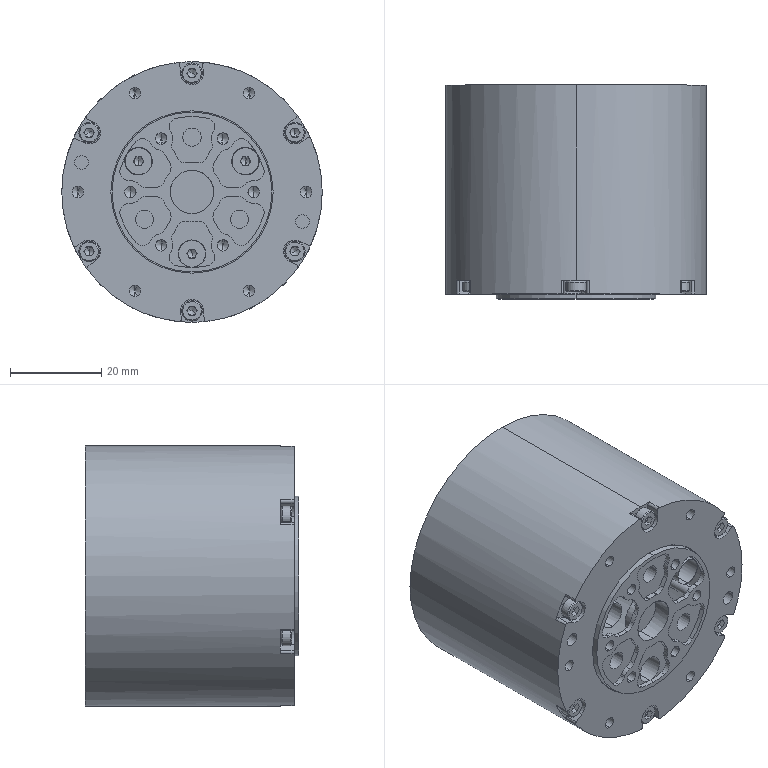Part | SolidWorks | features BaseBody 1 | 1 solid | 699 faces | box 57 x 46.8 x 57 mm | volume 109300 mm3 | cylinder 325 | plane 197 | cone 96 | spline 75 | torus 6 | commonest cylinder face diameters 2.28 x72 4 x54 2.5 x50 2.05 x38 5 x24 1 x12